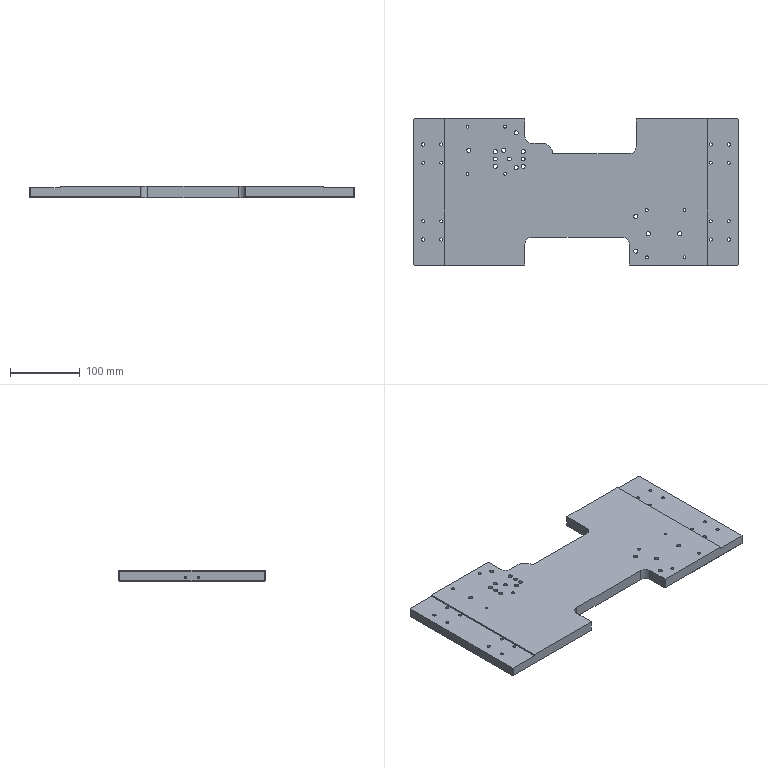NC program | NX | posted with a generic post | part box 467 x 210 x 16 mm
Whole program, first 1630 of 1789 lines:
N10 G17 G21 G94 G90
(FLOOR_WALL , TOOL : D63)
N12 T01 M6
N14 G54
N16 G17 G0 G90 X-271. Y107.997 S6500 M3
N18 G43 Z30. H1
N20 Z3.
N22 G94 G1 Z0. F1250.
N24 X-268.
N26 X268.
N28 Y80.74
N30 X-268.
N32 Y53.484
N34 X268.
N36 Y26.227
N38 X-268.
N40 Y-1.03
N42 X268.
N44 Y-28.287
N46 X-268.
N48 Y-55.543
N50 X268.
N52 Y-82.8
N54 X-268.
N56 X-271.
N58 Z3.
N60 G0 Z30.
N62 M5
(DRILLING_COPY_1 , TOOL : D6A45)
N64 T07 M6
N66 G54
N68 G17 G0 G90 X141.5 Y-65. S3000 M3
N70 G43 Z30. H7
N72 G94 G81 G98 Z-2.1 F200. R3.
N74 X193.5 Y-68.3
N76 X196.5 Y-99.
N78 X225.5
N80 X219.5 Y-68.3
N82 Y-42.3
N84 X225.5 Y-31.
N86 X193.5 Y-42.3
N88 X196.5 Y-31.
N90 X193.5 Y42.3
N92 X219.5
N94 Y68.3
N96 X193.5
N98 X156. Y94.
N100 X154. Y60.
N102 X156. Y26.
N104 X141.5 Y5.
N106 X91.5
N108 X102. Y26.
N110 X116. Y37.
N112 Y47.5
N114 Y58.
N116 X102. Y94.
N118 X86. Y85.
N120 X104. Y60.
N122 X96. Y47.5
N124 X86. Y35.
N126 X76. Y37.
N128 Y47.5
N130 Y58.
N132 X-8.5 Y5.
N134 X-108.5
N136 X-102. Y-26.
N138 X-86. Y-35.
N140 X-104. Y-60.
N142 X-86. Y-85.
N144 X-102. Y-94.
N146 X-156.
N148 X-149. Y-60.
N150 X-156. Y-26.
N152 X-193.5 Y-42.3
N154 Y-68.3
N156 X-219.5
N158 Y-42.3
N160 X-208.5 Y5.
N162 X-219.5 Y42.3
N164 Y68.3
N166 X-193.5
N168 Y42.3
N170 G80
N172 G0 X-193.5 Y42.3 Z30.
N174 M5
(DRILLING_COPY_1_COPY_COPY_COPY_COPY , TOOL : 4.5ZT)
N176 T19 M6
N178 G54
N180 G17 G0 G90 X-193.5 Y-68.3 S2000 M3
N182 G43 Z30. H19
N184 G94 G83 G98 Z-15.852 F150. Q2. R3.
N186 X-219.5
N188 Y-42.3
N190 X-193.5
N192 Y42.3
N194 X-219.5
N196 Y68.3
N198 X-193.5
N200 X193.5
N202 X219.5
N204 Y42.3
N206 X193.5
N208 Y-42.3
N210 Y-68.3
N212 X219.5
N214 Y-42.3
N216 G80
N218 G0 X219.5 Y-42.3 Z30.
N220 M5
(DRILLING_COPY_1_COPY_COPY_1 , TOOL : 5.8ZT)
N222 T18 M6
N224 G54
N226 G17 G0 G90 X-149. Y-60. S2000 M3
N228 G43 Z30. H18
N230 G94 G83 G98 Z-19.242 F120. Q2. R3.
N232 X-104.
N234 X-86. Y-85.
N236 Y-35.
N238 X76. Y37.
N240 X86. Y35.
N242 X76. Y58.
N244 X86. Y85.
N246 X104. Y60.
N248 X116. Y58.
N250 Y37.
N252 X154. Y60.
N254 G80
N256 G0 X154. Y60. Z30.
N258 M5
(DRILLING_COPY_1_COPY_COPY_1_COPY , TOOL : 6.0JD)
N260 T20 M6
N262 G54
N264 G17 G0 G90 X-149. Y-60. S1000 M3
N266 G43 Z30. H20
N268 G94 G85 G98 Z-16.5 F40. R3.
N270 X-104.
N272 X-86. Y-85.
N274 Y-35.
N276 X76. Y37.
N278 X86. Y35.
N280 X76. Y58.
N282 X86. Y85.
N284 X104. Y60.
N286 X116. Y58.
N288 Y37.
N290 X154. Y60.
N292 G80
N294 G0 X154. Y60. Z30.
N296 M5
(DRILLING_COPY_1_COPY_COPY_1_COPY_1 , TOOL : 5.5ZT)
N298 T12 M6
N300 G54
N302 G17 G0 G90 X76. Y47.5 S2000 M3
N304 G43 Z30. H12
N306 G94 G83 G98 Z-19.152 F120. Q2. R3.
N308 X96.
N310 X116.
N312 G80
N314 G0 X116. Y47.5 Z30.
N316 M5
(DRILLING_COPY_1_COPY , TOOL : 4.2ZT)
N318 T14 M6
N320 G54
N322 G17 G0 G90 X102. Y94. S2000 M3
N324 G43 Z30. H14
N326 G94 G83 G98 Z-18.762 F150. Q2. R3.
N328 X156.
N330 Y26.
N332 X102.
N334 X-102. Y-26.
N336 X-156.
N338 Y-94.
N340 X-102.
N342 G80
N344 G0 X-102. Y-94. Z30.
N346 M5
(DRILLING_COPY_1_COPY_COPY_COPY_COPY_COPY , TOOL : 3.3ZT)
N348 T13 M6
N350 G54
N352 G17 G0 G90 X141.5 Y-65. S2000 M3
N354 G43 Z30. H13
N356 G94 G83 G98 Z-11.091 F150. Q2. R3.
N358 X196.5 Y-99. Z-9.091
N360 X225.5
N362 Y-31.
N364 X196.5
N366 X141.5 Y5. Z-11.091
N368 X91.5
N370 X-8.5
N372 X-108.5
N374 X-208.5
N376 G80
N378 G0 X-208.5 Y5. Z30.
N380 M5
(ZLEVEL_PROFILE , TOOL : D10)
N382 T10 M6
N384 G54
N386 G17 G0 G90 X-238.6 Y-46.987 S7000 M3
N388 G43 Z30. H10
N390 Z1.5
N392 G94 G1 Y0. Z-0.963 F1000.
N394 Y104. F3000.
N396 G2 X-237.106 Y107.606 R5.1
N398 G1 X-236.106 Y108.606
N400 G2 X-232.5 Y110.1 R5.1
N402 G1 X-86.5
N404 G2 X-81.4 Y105. R5.1
N406 G1 Y65.
N408 G3 X-76.5 Y60.1 R4.9
N410 G1 X28.401
N412 G2 X29.894 Y63.606 R5.1
N414 G1 X39.894 Y73.606
N416 G2 X43.5 Y75.1 R5.1
N418 G1 X63.5
N420 G3 X68.4 Y80. R4.9
N422 G1 Y105.
N424 G2 X73.5 Y110.1 R5.1
N426 G1 X232.5
N428 G2 X236.106 Y108.606 R5.1
N430 G1 X237.106 Y107.606
N432 G2 X238.6 Y104. R5.1
N434 G1 Y-104.
N436 G2 X237.106 Y-107.606 R5.1
N438 G1 X236.106 Y-108.606
N440 G2 X232.5 Y-110.1 R5.1
N442 G1 X73.5
N444 G2 X68.4 Y-105. R5.1
N446 G1 Y-75.
N448 G3 X63.5 Y-70.1 R4.9
N450 G1 X-66.5
N452 G3 X-71.4 Y-75. R4.9
N454 G1 Y-105.
N456 G2 X-76.5 Y-110.1 R5.1
N458 G1 X-232.5
N460 G2 X-236.106 Y-108.606 R5.1
N462 G1 X-237.106 Y-107.606
N464 G2 X-238.6 Y-104. R5.1
N466 G1 Y0.
N468 Y55.142 Z-1.925
N470 Y104.
N472 G2 X-237.106 Y107.606 R5.1
N474 G1 X-236.106 Y108.606
N476 G2 X-232.5 Y110.1 R5.1
N478 G1 X-86.5
N480 G2 X-81.4 Y105. R5.1
N482 G1 Y65.
N484 G3 X-76.5 Y60.1 R4.9
N486 G1 X28.401
N488 G2 X29.894 Y63.606 R5.1
N490 G1 X39.894 Y73.606
N492 G2 X43.5 Y75.1 R5.1
N494 G1 X63.5
N496 G3 X68.4 Y80. R4.9
N498 G1 Y105.
N500 G2 X73.5 Y110.1 R5.1
N502 G1 X232.5
N504 G2 X236.106 Y108.606 R5.1
N506 G1 X237.106 Y107.606
N508 G2 X238.6 Y104. R5.1
N510 G1 Y-104.
N512 G2 X237.106 Y-107.606 R5.1
N514 G1 X236.106 Y-108.606
N516 G2 X232.5 Y-110.1 R5.1
N518 G1 X73.5
N520 G2 X68.4 Y-105. R5.1
N522 G1 Y-75.
N524 G3 X63.5 Y-70.1 R4.9
N526 G1 X-66.5
N528 G3 X-71.4 Y-75. R4.9
N530 G1 Y-105.
N532 G2 X-76.5 Y-110.1 R5.1
N534 G1 X-232.5
N536 G2 X-236.106 Y-108.606 R5.1
N538 G1 X-237.106 Y-107.606
N540 G2 X-238.6 Y-104. R5.1
N542 G1 Y0.
N544 Y55.142 Z-2.888
N546 Y104.
N548 G2 X-237.106 Y107.606 R5.1
N550 G1 X-236.106 Y108.606
N552 G2 X-232.5 Y110.1 R5.1
N554 G1 X-86.5
N556 G2 X-81.4 Y105. R5.1
N558 G1 Y65.
N560 G3 X-76.5 Y60.1 R4.9
N562 G1 X28.401
N564 G2 X29.894 Y63.606 R5.1
N566 G1 X39.894 Y73.606
N568 G2 X43.5 Y75.1 R5.1
N570 G1 X63.5
N572 G3 X68.4 Y80. R4.9
N574 G1 Y105.
N576 G2 X73.5 Y110.1 R5.1
N578 G1 X232.5
N580 G2 X236.106 Y108.606 R5.1
N582 G1 X237.106 Y107.606
N584 G2 X238.6 Y104. R5.1
N586 G1 Y-104.
N588 G2 X237.106 Y-107.606 R5.1
N590 G1 X236.106 Y-108.606
N592 G2 X232.5 Y-110.1 R5.1
N594 G1 X73.5
N596 G2 X68.4 Y-105. R5.1
N598 G1 Y-75.
N600 G3 X63.5 Y-70.1 R4.9
N602 G1 X-66.5
N604 G3 X-71.4 Y-75. R4.9
N606 G1 Y-105.
N608 G2 X-76.5 Y-110.1 R5.1
N610 G1 X-232.5
N612 G2 X-236.106 Y-108.606 R5.1
N614 G1 X-237.106 Y-107.606
N616 G2 X-238.6 Y-104. R5.1
N618 G1 Y0.
N620 Y55.142 Z-3.85
N622 Y104.
N624 G2 X-237.106 Y107.606 R5.1
N626 G1 X-236.106 Y108.606
N628 G2 X-232.5 Y110.1 R5.1
N630 G1 X-86.5
N632 G2 X-81.4 Y105. R5.1
N634 G1 Y65.
N636 G3 X-76.5 Y60.1 R4.9
N638 G1 X28.401
N640 G2 X29.894 Y63.606 R5.1
N642 G1 X39.894 Y73.606
N644 G2 X43.5 Y75.1 R5.1
N646 G1 X63.5
N648 G3 X68.4 Y80. R4.9
N650 G1 Y105.
N652 G2 X73.5 Y110.1 R5.1
N654 G1 X232.5
N656 G2 X236.106 Y108.606 R5.1
N658 G1 X237.106 Y107.606
N660 G2 X238.6 Y104. R5.1
N662 G1 Y-104.
N664 G2 X237.106 Y-107.606 R5.1
N666 G1 X236.106 Y-108.606
N668 G2 X232.5 Y-110.1 R5.1
N670 G1 X73.5
N672 G2 X68.4 Y-105. R5.1
N674 G1 Y-75.
N676 G3 X63.5 Y-70.1 R4.9
N678 G1 X-66.5
N680 G3 X-71.4 Y-75. R4.9
N682 G1 Y-105.
N684 G2 X-76.5 Y-110.1 R5.1
N686 G1 X-232.5
N688 G2 X-236.106 Y-108.606 R5.1
N690 G1 X-237.106 Y-107.606
N692 G2 X-238.6 Y-104. R5.1
N694 G1 Y0.
N696 Y55.142 Z-4.813
N698 Y104.
N700 G2 X-237.106 Y107.606 R5.1
N702 G1 X-236.106 Y108.606
N704 G2 X-232.5 Y110.1 R5.1
N706 G1 X-86.5
N708 G2 X-81.4 Y105. R5.1
N710 G1 Y65.
N712 G3 X-76.5 Y60.1 R4.9
N714 G1 X28.401
N716 G2 X29.894 Y63.606 R5.1
N718 G1 X39.894 Y73.606
N720 G2 X43.5 Y75.1 R5.1
N722 G1 X63.5
N724 G3 X68.4 Y80. R4.9
N726 G1 Y105.
N728 G2 X73.5 Y110.1 R5.1
N730 G1 X232.5
N732 G2 X236.106 Y108.606 R5.1
N734 G1 X237.106 Y107.606
N736 G2 X238.6 Y104. R5.1
N738 G1 Y-104.
N740 G2 X237.106 Y-107.606 R5.1
N742 G1 X236.106 Y-108.606
N744 G2 X232.5 Y-110.1 R5.1
N746 G1 X73.5
N748 G2 X68.4 Y-105. R5.1
N750 G1 Y-75.
N752 G3 X63.5 Y-70.1 R4.9
N754 G1 X-66.5
N756 G3 X-71.4 Y-75. R4.9
N758 G1 Y-105.
N760 G2 X-76.5 Y-110.1 R5.1
N762 G1 X-232.5
N764 G2 X-236.106 Y-108.606 R5.1
N766 G1 X-237.106 Y-107.606
N768 G2 X-238.6 Y-104. R5.1
N770 G1 Y0.
N772 Y55.142 Z-5.775
N774 Y104.
N776 G2 X-237.106 Y107.606 R5.1
N778 G1 X-236.106 Y108.606
N780 G2 X-232.5 Y110.1 R5.1
N782 G1 X-86.5
N784 G2 X-81.4 Y105. R5.1
N786 G1 Y65.
N788 G3 X-76.5 Y60.1 R4.9
N790 G1 X28.401
N792 G2 X29.894 Y63.606 R5.1
N794 G1 X39.894 Y73.606
N796 G2 X43.5 Y75.1 R5.1
N798 G1 X63.5
N800 G3 X68.4 Y80. R4.9
N802 G1 Y105.
N804 G2 X73.5 Y110.1 R5.1
N806 G1 X232.5
N808 G2 X236.106 Y108.606 R5.1
N810 G1 X237.106 Y107.606
N812 G2 X238.6 Y104. R5.1
N814 G1 Y-104.
N816 G2 X237.106 Y-107.606 R5.1
N818 G1 X236.106 Y-108.606
N820 G2 X232.5 Y-110.1 R5.1
N822 G1 X73.5
N824 G2 X68.4 Y-105. R5.1
N826 G1 Y-75.
N828 G3 X63.5 Y-70.1 R4.9
N830 G1 X-66.5
N832 G3 X-71.4 Y-75. R4.9
N834 G1 Y-105.
N836 G2 X-76.5 Y-110.1 R5.1
N838 G1 X-232.5
N840 G2 X-236.106 Y-108.606 R5.1
N842 G1 X-237.106 Y-107.606
N844 G2 X-238.6 Y-104. R5.1
N846 G1 Y0.
N848 Y55.142 Z-6.738
N850 Y104.
N852 G2 X-237.106 Y107.606 R5.1
N854 G1 X-236.106 Y108.606
N856 G2 X-232.5 Y110.1 R5.1
N858 G1 X-86.5
N860 G2 X-81.4 Y105. R5.1
N862 G1 Y65.
N864 G3 X-76.5 Y60.1 R4.9
N866 G1 X28.401
N868 G2 X29.894 Y63.606 R5.1
N870 G1 X39.894 Y73.606
N872 G2 X43.5 Y75.1 R5.1
N874 G1 X63.5
N876 G3 X68.4 Y80. R4.9
N878 G1 Y105.
N880 G2 X73.5 Y110.1 R5.1
N882 G1 X232.5
N884 G2 X236.106 Y108.606 R5.1
N886 G1 X237.106 Y107.606
N888 G2 X238.6 Y104. R5.1
N890 G1 Y-104.
N892 G2 X237.106 Y-107.606 R5.1
N894 G1 X236.106 Y-108.606
N896 G2 X232.5 Y-110.1 R5.1
N898 G1 X73.5
N900 G2 X68.4 Y-105. R5.1
N902 G1 Y-75.
N904 G3 X63.5 Y-70.1 R4.9
N906 G1 X-66.5
N908 G3 X-71.4 Y-75. R4.9
N910 G1 Y-105.
N912 G2 X-76.5 Y-110.1 R5.1
N914 G1 X-232.5
N916 G2 X-236.106 Y-108.606 R5.1
N918 G1 X-237.106 Y-107.606
N920 G2 X-238.6 Y-104. R5.1
N922 G1 Y0.
N924 Y55.142 Z-7.7
N926 Y104.
N928 G2 X-237.106 Y107.606 R5.1
N930 G1 X-236.106 Y108.606
N932 G2 X-232.5 Y110.1 R5.1
N934 G1 X-86.5
N936 G2 X-81.4 Y105. R5.1
N938 G1 Y65.
N940 G3 X-76.5 Y60.1 R4.9
N942 G1 X28.401
N944 G2 X29.894 Y63.606 R5.1
N946 G1 X39.894 Y73.606
N948 G2 X43.5 Y75.1 R5.1
N950 G1 X63.5
N952 G3 X68.4 Y80. R4.9
N954 G1 Y105.
N956 G2 X73.5 Y110.1 R5.1
N958 G1 X232.5
N960 G2 X236.106 Y108.606 R5.1
N962 G1 X237.106 Y107.606
N964 G2 X238.6 Y104. R5.1
N966 G1 Y-104.
N968 G2 X237.106 Y-107.606 R5.1
N970 G1 X236.106 Y-108.606
N972 G2 X232.5 Y-110.1 R5.1
N974 G1 X73.5
N976 G2 X68.4 Y-105. R5.1
N978 G1 Y-75.
N980 G3 X63.5 Y-70.1 R4.9
N982 G1 X-66.5
N984 G3 X-71.4 Y-75. R4.9
N986 G1 Y-105.
N988 G2 X-76.5 Y-110.1 R5.1
N990 G1 X-232.5
N992 G2 X-236.106 Y-108.606 R5.1
N994 G1 X-237.106 Y-107.606
N996 G2 X-238.6 Y-104. R5.1
N998 G1 Y0.
N1000 Y55.142 Z-8.663
N1002 Y104.
N1004 G2 X-237.106 Y107.606 R5.1
N1006 G1 X-236.106 Y108.606
N1008 G2 X-232.5 Y110.1 R5.1
N1010 G1 X-86.5
N1012 G2 X-81.4 Y105. R5.1
N1014 G1 Y65.
N1016 G3 X-76.5 Y60.1 R4.9
N1018 G1 X28.401
N1020 G2 X29.894 Y63.606 R5.1
N1022 G1 X39.894 Y73.606
N1024 G2 X43.5 Y75.1 R5.1
N1026 G1 X63.5
N1028 G3 X68.4 Y80. R4.9
N1030 G1 Y105.
N1032 G2 X73.5 Y110.1 R5.1
N1034 G1 X232.5
N1036 G2 X236.106 Y108.606 R5.1
N1038 G1 X237.106 Y107.606
N1040 G2 X238.6 Y104. R5.1
N1042 G1 Y-104.
N1044 G2 X237.106 Y-107.606 R5.1
N1046 G1 X236.106 Y-108.606
N1048 G2 X232.5 Y-110.1 R5.1
N1050 G1 X73.5
N1052 G2 X68.4 Y-105. R5.1
N1054 G1 Y-75.
N1056 G3 X63.5 Y-70.1 R4.9
N1058 G1 X-66.5
N1060 G3 X-71.4 Y-75. R4.9
N1062 G1 Y-105.
N1064 G2 X-76.5 Y-110.1 R5.1
N1066 G1 X-232.5
N1068 G2 X-236.106 Y-108.606 R5.1
N1070 G1 X-237.106 Y-107.606
N1072 G2 X-238.6 Y-104. R5.1
N1074 G1 Y0.
N1076 Y55.142 Z-9.625
N1078 Y104.
N1080 G2 X-237.106 Y107.606 R5.1
N1082 G1 X-236.106 Y108.606
N1084 G2 X-232.5 Y110.1 R5.1
N1086 G1 X-86.5
N1088 G2 X-81.4 Y105. R5.1
N1090 G1 Y65.
N1092 G3 X-76.5 Y60.1 R4.9
N1094 G1 X28.401
N1096 G2 X29.894 Y63.606 R5.1
N1098 G1 X39.894 Y73.606
N1100 G2 X43.5 Y75.1 R5.1
N1102 G1 X63.5
N1104 G3 X68.4 Y80. R4.9
N1106 G1 Y105.
N1108 G2 X73.5 Y110.1 R5.1
N1110 G1 X232.5
N1112 G2 X236.106 Y108.606 R5.1
N1114 G1 X237.106 Y107.606
N1116 G2 X238.6 Y104. R5.1
N1118 G1 Y-104.
N1120 G2 X237.106 Y-107.606 R5.1
N1122 G1 X236.106 Y-108.606
N1124 G2 X232.5 Y-110.1 R5.1
N1126 G1 X73.5
N1128 G2 X68.4 Y-105. R5.1
N1130 G1 Y-75.
N1132 G3 X63.5 Y-70.1 R4.9
N1134 G1 X-66.5
N1136 G3 X-71.4 Y-75. R4.9
N1138 G1 Y-105.
N1140 G2 X-76.5 Y-110.1 R5.1
N1142 G1 X-232.5
N1144 G2 X-236.106 Y-108.606 R5.1
N1146 G1 X-237.106 Y-107.606
N1148 G2 X-238.6 Y-104. R5.1
N1150 G1 Y0.
N1152 Y55.142 Z-10.588
N1154 Y104.
N1156 G2 X-237.106 Y107.606 R5.1
N1158 G1 X-236.106 Y108.606
N1160 G2 X-232.5 Y110.1 R5.1
N1162 G1 X-86.5
N1164 G2 X-81.4 Y105. R5.1
N1166 G1 Y65.
N1168 G3 X-76.5 Y60.1 R4.9
N1170 G1 X28.401
N1172 G2 X29.894 Y63.606 R5.1
N1174 G1 X39.894 Y73.606
N1176 G2 X43.5 Y75.1 R5.1
N1178 G1 X63.5
N1180 G3 X68.4 Y80. R4.9
N1182 G1 Y105.
N1184 G2 X73.5 Y110.1 R5.1
N1186 G1 X232.5
N1188 G2 X236.106 Y108.606 R5.1
N1190 G1 X237.106 Y107.606
N1192 G2 X238.6 Y104. R5.1
N1194 G1 Y-104.
N1196 G2 X237.106 Y-107.606 R5.1
N1198 G1 X236.106 Y-108.606
N1200 G2 X232.5 Y-110.1 R5.1
N1202 G1 X73.5
N1204 G2 X68.4 Y-105. R5.1
N1206 G1 Y-75.
N1208 G3 X63.5 Y-70.1 R4.9
N1210 G1 X-66.5
N1212 G3 X-71.4 Y-75. R4.9
N1214 G1 Y-105.
N1216 G2 X-76.5 Y-110.1 R5.1
N1218 G1 X-232.5
N1220 G2 X-236.106 Y-108.606 R5.1
N1222 G1 X-237.106 Y-107.606
N1224 G2 X-238.6 Y-104. R5.1
N1226 G1 Y0.
N1228 Y55.142 Z-11.55
N1230 Y104.
N1232 G2 X-237.106 Y107.606 R5.1
N1234 G1 X-236.106 Y108.606
N1236 G2 X-232.5 Y110.1 R5.1
N1238 G1 X-86.5
N1240 G2 X-81.4 Y105. R5.1
N1242 G1 Y65.
N1244 G3 X-76.5 Y60.1 R4.9
N1246 G1 X28.401
N1248 G2 X29.894 Y63.606 R5.1
N1250 G1 X39.894 Y73.606
N1252 G2 X43.5 Y75.1 R5.1
N1254 G1 X63.5
N1256 G3 X68.4 Y80. R4.9
N1258 G1 Y105.
N1260 G2 X73.5 Y110.1 R5.1
N1262 G1 X232.5
N1264 G2 X236.106 Y108.606 R5.1
N1266 G1 X237.106 Y107.606
N1268 G2 X238.6 Y104. R5.1
N1270 G1 Y-104.
N1272 G2 X237.106 Y-107.606 R5.1
N1274 G1 X236.106 Y-108.606
N1276 G2 X232.5 Y-110.1 R5.1
N1278 G1 X73.5
N1280 G2 X68.4 Y-105. R5.1
N1282 G1 Y-75.
N1284 G3 X63.5 Y-70.1 R4.9
N1286 G1 X-66.5
N1288 G3 X-71.4 Y-75. R4.9
N1290 G1 Y-105.
N1292 G2 X-76.5 Y-110.1 R5.1
N1294 G1 X-232.5
N1296 G2 X-236.106 Y-108.606 R5.1
N1298 G1 X-237.106 Y-107.606
N1300 G2 X-238.6 Y-104. R5.1
N1302 G1 Y0.
N1304 Y55.142 Z-12.513
N1306 Y104.
N1308 G2 X-237.106 Y107.606 R5.1
N1310 G1 X-236.106 Y108.606
N1312 G2 X-232.5 Y110.1 R5.1
N1314 G1 X-86.5
N1316 G2 X-81.4 Y105. R5.1
N1318 G1 Y65.
N1320 G3 X-76.5 Y60.1 R4.9
N1322 G1 X28.401
N1324 G2 X29.894 Y63.606 R5.1
N1326 G1 X39.894 Y73.606
N1328 G2 X43.5 Y75.1 R5.1
N1330 G1 X63.5
N1332 G3 X68.4 Y80. R4.9
N1334 G1 Y105.
N1336 G2 X73.5 Y110.1 R5.1
N1338 G1 X232.5
N1340 G2 X236.106 Y108.606 R5.1
N1342 G1 X237.106 Y107.606
N1344 G2 X238.6 Y104. R5.1
N1346 G1 Y-104.
N1348 G2 X237.106 Y-107.606 R5.1
N1350 G1 X236.106 Y-108.606
N1352 G2 X232.5 Y-110.1 R5.1
N1354 G1 X73.5
N1356 G2 X68.4 Y-105. R5.1
N1358 G1 Y-75.
N1360 G3 X63.5 Y-70.1 R4.9
N1362 G1 X-66.5
N1364 G3 X-71.4 Y-75. R4.9
N1366 G1 Y-105.
N1368 G2 X-76.5 Y-110.1 R5.1
N1370 G1 X-232.5
N1372 G2 X-236.106 Y-108.606 R5.1
N1374 G1 X-237.106 Y-107.606
N1376 G2 X-238.6 Y-104. R5.1
N1378 G1 Y0.
N1380 Y55.142 Z-13.475
N1382 Y104.
N1384 G2 X-237.106 Y107.606 R5.1
N1386 G1 X-236.106 Y108.606
N1388 G2 X-232.5 Y110.1 R5.1
N1390 G1 X-86.5
N1392 G2 X-81.4 Y105. R5.1
N1394 G1 Y65.
N1396 G3 X-76.5 Y60.1 R4.9
N1398 G1 X28.401
N1400 G2 X29.894 Y63.606 R5.1
N1402 G1 X39.894 Y73.606
N1404 G2 X43.5 Y75.1 R5.1
N1406 G1 X63.5
N1408 G3 X68.4 Y80. R4.9
N1410 G1 Y105.
N1412 G2 X73.5 Y110.1 R5.1
N1414 G1 X232.5
N1416 G2 X236.106 Y108.606 R5.1
N1418 G1 X237.106 Y107.606
N1420 G2 X238.6 Y104. R5.1
N1422 G1 Y-104.
N1424 G2 X237.106 Y-107.606 R5.1
N1426 G1 X236.106 Y-108.606
N1428 G2 X232.5 Y-110.1 R5.1
N1430 G1 X73.5
N1432 G2 X68.4 Y-105. R5.1
N1434 G1 Y-75.
N1436 G3 X63.5 Y-70.1 R4.9
N1438 G1 X-66.5
N1440 G3 X-71.4 Y-75. R4.9
N1442 G1 Y-105.
N1444 G2 X-76.5 Y-110.1 R5.1
N1446 G1 X-232.5
N1448 G2 X-236.106 Y-108.606 R5.1
N1450 G1 X-237.106 Y-107.606
N1452 G2 X-238.6 Y-104. R5.1
N1454 G1 Y0.
N1456 Y55.142 Z-14.438
N1458 Y104.
N1460 G2 X-237.106 Y107.606 R5.1
N1462 G1 X-236.106 Y108.606
N1464 G2 X-232.5 Y110.1 R5.1
N1466 G1 X-86.5
N1468 G2 X-81.4 Y105. R5.1
N1470 G1 Y65.
N1472 G3 X-76.5 Y60.1 R4.9
N1474 G1 X28.401
N1476 G2 X29.894 Y63.606 R5.1
N1478 G1 X39.894 Y73.606
N1480 G2 X43.5 Y75.1 R5.1
N1482 G1 X63.5
N1484 G3 X68.4 Y80. R4.9
N1486 G1 Y105.
N1488 G2 X73.5 Y110.1 R5.1
N1490 G1 X232.5
N1492 G2 X236.106 Y108.606 R5.1
N1494 G1 X237.106 Y107.606
N1496 G2 X238.6 Y104. R5.1
N1498 G1 Y-104.
N1500 G2 X237.106 Y-107.606 R5.1
N1502 G1 X236.106 Y-108.606
N1504 G2 X232.5 Y-110.1 R5.1
N1506 G1 X73.5
N1508 G2 X68.4 Y-105. R5.1
N1510 G1 Y-75.
N1512 G3 X63.5 Y-70.1 R4.9
N1514 G1 X-66.5
N1516 G3 X-71.4 Y-75. R4.9
N1518 G1 Y-105.
N1520 G2 X-76.5 Y-110.1 R5.1
N1522 G1 X-232.5
N1524 G2 X-236.106 Y-108.606 R5.1
N1526 G1 X-237.106 Y-107.606
N1528 G2 X-238.6 Y-104. R5.1
N1530 G1 Y0.
N1532 Y55.142 Z-15.4
N1534 Y104.
N1536 G2 X-237.106 Y107.606 R5.1
N1538 G1 X-236.106 Y108.606
N1540 G2 X-232.5 Y110.1 R5.1
N1542 G1 X-86.5
N1544 G2 X-81.4 Y105. R5.1
N1546 G1 Y65.
N1548 G3 X-76.5 Y60.1 R4.9
N1550 G1 X28.401
N1552 G2 X29.894 Y63.606 R5.1
N1554 G1 X39.894 Y73.606
N1556 G2 X43.5 Y75.1 R5.1
N1558 G1 X63.5
N1560 G3 X68.4 Y80. R4.9
N1562 G1 Y105.
N1564 G2 X73.5 Y110.1 R5.1
N1566 G1 X232.5
N1568 G2 X236.106 Y108.606 R5.1
N1570 G1 X237.106 Y107.606
N1572 G2 X238.6 Y104. R5.1
N1574 G1 Y-104.
N1576 G2 X237.106 Y-107.606 R5.1
N1578 G1 X236.106 Y-108.606
N1580 G2 X232.5 Y-110.1 R5.1
N1582 G1 X73.5
N1584 G2 X68.4 Y-105. R5.1
N1586 G1 Y-75.
N1588 G3 X63.5 Y-70.1 R4.9
N1590 G1 X-66.5
N1592 G3 X-71.4 Y-75. R4.9
N1594 G1 Y-105.
N1596 G2 X-76.5 Y-110.1 R5.1
N1598 G1 X-232.5
N1600 G2 X-236.106 Y-108.606 R5.1
N1602 G1 X-237.106 Y-107.606
N1604 G2 X-238.6 Y-104. R5.1
N1606 G1 Y55.142
N1608 Z-13.9
N1610 G0 Z30.
N1612 M5
(HOLE_MILLING , TOOL : D6)
N1614 T06 M6
N1616 G54
N1618 G17 G0 G90 X-219.5 Y68.3 S7000 M3
N1620 G43 Z30. H6
N1622 Z0.5
N1624 G94 G3 X-220. Y68.8 R0.5 F1500.
N1626 X-220.5 Y68.3 R0.5
N1628 X-220.5 Y68.3 Z0. I1. J0.
N1630 X-220.5 Y68.3 Z-0.5 I1. J0.
N1632 X-220.5 Y68.3 Z-1. I1. J0.
N1634 X-220.5 Y68.3 Z-1.5 I1. J0.
N1636 X-220.5 Y68.3 Z-2. I1. J0.
N1638 X-220.5 Y68.3 Z-2.5 I1. J0.
N1640 X-220.5 Y68.3 Z-3. I1. J0.
N1642 X-220.5 Y68.3 Z-3.5 I1. J0.
N1644 X-220.5 Y68.3 Z-4. I1. J0.
N1646 X-219.809 Y69.251 Z-4.4 R-1.
N1648 X-220.451 Y67.991 R1.
N1650 X-219.809 Y69.251 R-1.
N1652 X-220.13 Y68.621 R0.5
N1654 X-219.5 Y68.3 R0.5
N1656 G0 Z30.
N1658 X-193.5
N1660 Z0.5
N1662 G3 X-194. Y68.8 R0.5
N1664 X-194.5 Y68.3 R0.5
N1666 X-194.5 Y68.3 Z0. I1. J0.
N1668 X-194.5 Y68.3 Z-0.5 I1. J0.
N1670 X-194.5 Y68.3 Z-1. I1. J0.
N1672 X-194.5 Y68.3 Z-1.5 I1. J0.
N1674 X-194.5 Y68.3 Z-2. I1. J0.
N1676 X-194.5 Y68.3 Z-2.5 I1. J0.
N1678 X-194.5 Y68.3 Z-3. I1. J0.
N1680 X-194.5 Y68.3 Z-3.5 I1. J0.
N1682 X-194.5 Y68.3 Z-4. I1. J0.
N1684 X-193.809 Y69.251 Z-4.4 R-1.
N1686 X-194.451 Y67.991 R1.
N1688 X-193.809 Y69.251 R-1.
N1690 X-194.13 Y68.621 R0.5
N1692 X-193.5 Y68.3 R0.5
N1694 G0 Z30.
N1696 Y42.3
N1698 Z0.5
N1700 G3 X-194. Y42.8 R0.5
N1702 X-194.5 Y42.3 R0.5
N1704 X-194.5 Y42.3 Z0. I1. J0.
N1706 X-194.5 Y42.3 Z-0.5 I1. J0.
N1708 X-194.5 Y42.3 Z-1. I1. J0.
N1710 X-194.5 Y42.3 Z-1.5 I1. J0.
N1712 X-194.5 Y42.3 Z-2. I1. J0.
N1714 X-194.5 Y42.3 Z-2.5 I1. J0.
N1716 X-194.5 Y42.3 Z-3. I1. J0.
N1718 X-194.5 Y42.3 Z-3.5 I1. J0.
N1720 X-194.5 Y42.3 Z-4. I1. J0.
N1722 X-193.809 Y43.251 Z-4.4 R-1.
N1724 X-194.451 Y41.991 R1.
N1726 X-193.809 Y43.251 R-1.
N1728 X-194.13 Y42.621 R0.5
N1730 X-193.5 Y42.3 R0.5
N1732 G0 Z30.
N1734 X-219.5
N1736 Z0.5
N1738 G3 X-220. Y42.8 R0.5
N1740 X-220.5 Y42.3 R0.5
N1742 X-220.5 Y42.3 Z0. I1. J0.
N1744 X-220.5 Y42.3 Z-0.5 I1. J0.
N1746 X-220.5 Y42.3 Z-1. I1. J0.
N1748 X-220.5 Y42.3 Z-1.5 I1. J0.
N1750 X-220.5 Y42.3 Z-2. I1. J0.
N1752 X-220.5 Y42.3 Z-2.5 I1. J0.
N1754 X-220.5 Y42.3 Z-3. I1. J0.
N1756 X-220.5 Y42.3 Z-3.5 I1. J0.
N1758 X-220.5 Y42.3 Z-4. I1. J0.
N1760 X-219.809 Y43.251 Z-4.4 R-1.
N1762 X-220.451 Y41.991 R1.
N1764 X-219.809 Y43.251 R-1.
N1766 X-220.13 Y42.621 R0.5
N1768 X-219.5 Y42.3 R0.5
N1770 G0 Z30.
N1772 Y-42.3
N1774 Z0.5
N1776 G3 X-220. Y-41.8 R0.5
N1778 X-220.5 Y-42.3 R0.5
N1780 X-220.5 Y-42.3 Z0. I1. J0.
N1782 X-220.5 Y-42.3 Z-0.5 I1. J0.
N1784 X-220.5 Y-42.3 Z-1. I1. J0.
N1786 X-220.5 Y-42.3 Z-1.5 I1. J0.
N1788 X-220.5 Y-42.3 Z-2. I1. J0.
N1790 X-220.5 Y-42.3 Z-2.5 I1. J0.
N1792 X-220.5 Y-42.3 Z-3. I1. J0.
N1794 X-220.5 Y-42.3 Z-3.5 I1. J0.
N1796 X-220.5 Y-42.3 Z-4. I1. J0.
N1798 X-219.809 Y-41.349 Z-4.4 R-1.
N1800 X-220.451 Y-42.609 R1.
N1802 X-219.809 Y-41.349 R-1.
N1804 X-220.13 Y-41.979 R0.5
N1806 X-219.5 Y-42.3 R0.5
N1808 G0 Z30.
N1810 Y-68.3
N1812 Z0.5
N1814 G3 X-220. Y-67.8 R0.5
N1816 X-220.5 Y-68.3 R0.5
N1818 X-220.5 Y-68.3 Z0. I1. J0.
N1820 X-220.5 Y-68.3 Z-0.5 I1. J0.
N1822 X-220.5 Y-68.3 Z-1. I1. J0.
N1824 X-220.5 Y-68.3 Z-1.5 I1. J0.
N1826 X-220.5 Y-68.3 Z-2. I1. J0.
N1828 X-220.5 Y-68.3 Z-2.5 I1. J0.
N1830 X-220.5 Y-68.3 Z-3. I1. J0.
N1832 X-220.5 Y-68.3 Z-3.5 I1. J0.
N1834 X-220.5 Y-68.3 Z-4. I1. J0.
N1836 X-219.809 Y-67.349 Z-4.4 R-1.
N1838 X-220.451 Y-68.609 R1.
N1840 X-219.809 Y-67.349 R-1.
N1842 X-220.13 Y-67.979 R0.5
N1844 X-219.5 Y-68.3 R0.5
N1846 G0 Z30.
N1848 X-193.5
N1850 Z0.5
N1852 G3 X-194. Y-67.8 R0.5
N1854 X-194.5 Y-68.3 R0.5
N1856 X-194.5 Y-68.3 Z0. I1. J0.
N1858 X-194.5 Y-68.3 Z-0.5 I1. J0.
N1860 X-194.5 Y-68.3 Z-1. I1. J0.
N1862 X-194.5 Y-68.3 Z-1.5 I1. J0.
N1864 X-194.5 Y-68.3 Z-2. I1. J0.
N1866 X-194.5 Y-68.3 Z-2.5 I1. J0.
N1868 X-194.5 Y-68.3 Z-3. I1. J0.
N1870 X-194.5 Y-68.3 Z-3.5 I1. J0.
N1872 X-194.5 Y-68.3 Z-4. I1. J0.
N1874 X-193.809 Y-67.349 Z-4.4 R-1.
N1876 X-194.451 Y-68.609 R1.
N1878 X-193.809 Y-67.349 R-1.
N1880 X-194.13 Y-67.979 R0.5
N1882 X-193.5 Y-68.3 R0.5
N1884 G0 Z30.
N1886 Y-42.3
N1888 Z0.5
N1890 G3 X-194. Y-41.8 R0.5
N1892 X-194.5 Y-42.3 R0.5
N1894 X-194.5 Y-42.3 Z0. I1. J0.
N1896 X-194.5 Y-42.3 Z-0.5 I1. J0.
N1898 X-194.5 Y-42.3 Z-1. I1. J0.
N1900 X-194.5 Y-42.3 Z-1.5 I1. J0.
N1902 X-194.5 Y-42.3 Z-2. I1. J0.
N1904 X-194.5 Y-42.3 Z-2.5 I1. J0.
N1906 X-194.5 Y-42.3 Z-3. I1. J0.
N1908 X-194.5 Y-42.3 Z-3.5 I1. J0.
N1910 X-194.5 Y-42.3 Z-4. I1. J0.
N1912 X-193.809 Y-41.349 Z-4.4 R-1.
N1914 X-194.451 Y-42.609 R1.
N1916 X-193.809 Y-41.349 R-1.
N1918 X-194.13 Y-41.979 R0.5
N1920 X-193.5 Y-42.3 R0.5
N1922 G0 Z30.
N1924 X76. Y47.5
N1926 Z0.5
N1928 G3 X75. Y48.5 R1.
N1930 X74. Y47.5 R1.
N1932 X74. Y47.5 Z0. I2. J0.
N1934 X74. Y47.5 Z-0.5 I2. J0.
N1936 X74. Y47.5 Z-1. I2. J0.
N1938 X74. Y47.5 Z-1.5 I2. J0.
N1940 X74. Y47.5 Z-2. I2. J0.
N1942 X74. Y47.5 Z-2.5 I2. J0.
N1944 X74. Y47.5 Z-3. I2. J0.
N1946 X74. Y47.5 Z-3.5 I2. J0.
N1948 X74. Y47.5 Z-4. I2. J0.
N1950 X75.382 Y49.402 Z-4.4 R-2.
N1952 X74.098 Y46.882 R2.
N1954 X75.382 Y49.402 R-2.
N1956 X74.74 Y48.142 R1.
N1958 X76. Y47.5 R1.
N1960 G0 Z30.
N1962 X96.
N1964 Z0.5
N1966 G3 X95. Y48.5 R1.
N1968 X94. Y47.5 R1.
N1970 X94. Y47.5 Z0. I2. J0.
N1972 X94. Y47.5 Z-0.5 I2. J0.
N1974 X94. Y47.5 Z-1. I2. J0.
N1976 X94. Y47.5 Z-1.5 I2. J0.
N1978 X94. Y47.5 Z-2. I2. J0.
N1980 X94. Y47.5 Z-2.5 I2. J0.
N1982 X94. Y47.5 Z-3. I2. J0.
N1984 X94. Y47.5 Z-3.5 I2. J0.
N1986 X94. Y47.5 Z-4. I2. J0.
N1988 X95.382 Y49.402 Z-4.4 R-2.
N1990 X94.098 Y46.882 R2.
N1992 X95.382 Y49.402 R-2.
N1994 X94.74 Y48.142 R1.
N1996 X96. Y47.5 R1.
N1998 G0 Z30.
N2000 X116.
N2002 Z0.5
N2004 G3 X115. Y48.5 R1.
N2006 X114. Y47.5 R1.
N2008 X114. Y47.5 Z0. I2. J0.
N2010 X114. Y47.5 Z-0.5 I2. J0.
N2012 X114. Y47.5 Z-1. I2. J0.
N2014 X114. Y47.5 Z-1.5 I2. J0.
N2016 X114. Y47.5 Z-2. I2. J0.
N2018 X114. Y47.5 Z-2.5 I2. J0.
N2020 X114. Y47.5 Z-3. I2. J0.
N2022 X114. Y47.5 Z-3.5 I2. J0.
N2024 X114. Y47.5 Z-4. I2. J0.
N2026 X115.382 Y49.402 Z-4.4 R-2.
N2028 X114.098 Y46.882 R2.
N2030 X115.382 Y49.402 R-2.
N2032 X114.74 Y48.142 R1.
N2034 X116. Y47.5 R1.
N2036 G0 Z30.
N2038 X193.5 Y42.3
N2040 Z0.5
N2042 G3 X193. Y42.8 R0.5
N2044 X192.5 Y42.3 R0.5
N2046 X192.5 Y42.3 Z0. I1. J0.
N2048 X192.5 Y42.3 Z-0.5 I1. J0.
N2050 X192.5 Y42.3 Z-1. I1. J0.
N2052 X192.5 Y42.3 Z-1.5 I1. J0.
N2054 X192.5 Y42.3 Z-2. I1. J0.
N2056 X192.5 Y42.3 Z-2.5 I1. J0.
N2058 X192.5 Y42.3 Z-3. I1. J0.
N2060 X192.5 Y42.3 Z-3.5 I1. J0.
N2062 X192.5 Y42.3 Z-4. I1. J0.
N2064 X193.191 Y43.251 Z-4.4 R-1.
N2066 X192.549 Y41.991 R1.
N2068 X193.191 Y43.251 R-1.
N2070 X192.87 Y42.621 R0.5
N2072 X193.5 Y42.3 R0.5
N2074 G0 Z30.
N2076 Y68.3
N2078 Z0.5
N2080 G3 X193. Y68.8 R0.5
N2082 X192.5 Y68.3 R0.5
N2084 X192.5 Y68.3 Z0. I1. J0.
N2086 X192.5 Y68.3 Z-0.5 I1. J0.
N2088 X192.5 Y68.3 Z-1. I1. J0.
N2090 X192.5 Y68.3 Z-1.5 I1. J0.
N2092 X192.5 Y68.3 Z-2. I1. J0.
N2094 X192.5 Y68.3 Z-2.5 I1. J0.
N2096 X192.5 Y68.3 Z-3. I1. J0.
N2098 X192.5 Y68.3 Z-3.5 I1. J0.
N2100 X192.5 Y68.3 Z-4. I1. J0.
N2102 X193.191 Y69.251 Z-4.4 R-1.
N2104 X192.549 Y67.991 R1.
N2106 X193.191 Y69.251 R-1.
N2108 X192.87 Y68.621 R0.5
N2110 X193.5 Y68.3 R0.5
N2112 G0 Z30.
N2114 X219.5
N2116 Z0.5
N2118 G3 X219. Y68.8 R0.5
N2120 X218.5 Y68.3 R0.5
N2122 X218.5 Y68.3 Z0. I1. J0.
N2124 X218.5 Y68.3 Z-0.5 I1. J0.
N2126 X218.5 Y68.3 Z-1. I1. J0.
N2128 X218.5 Y68.3 Z-1.5 I1. J0.
N2130 X218.5 Y68.3 Z-2. I1. J0.
N2132 X218.5 Y68.3 Z-2.5 I1. J0.
N2134 X218.5 Y68.3 Z-3. I1. J0.
N2136 X218.5 Y68.3 Z-3.5 I1. J0.
N2138 X218.5 Y68.3 Z-4. I1. J0.
N2140 X219.191 Y69.251 Z-4.4 R-1.
N2142 X218.549 Y67.991 R1.
N2144 X219.191 Y69.251 R-1.
N2146 X218.87 Y68.621 R0.5
N2148 X219.5 Y68.3 R0.5
N2150 G0 Z30.
N2152 Y42.3
N2154 Z0.5
N2156 G3 X219. Y42.8 R0.5
N2158 X218.5 Y42.3 R0.5
N2160 X218.5 Y42.3 Z0. I1. J0.
N2162 X218.5 Y42.3 Z-0.5 I1. J0.
N2164 X218.5 Y42.3 Z-1. I1. J0.
N2166 X218.5 Y42.3 Z-1.5 I1. J0.
N2168 X218.5 Y42.3 Z-2. I1. J0.
N2170 X218.5 Y42.3 Z-2.5 I1. J0.
N2172 X218.5 Y42.3 Z-3. I1. J0.
N2174 X218.5 Y42.3 Z-3.5 I1. J0.
N2176 X218.5 Y42.3 Z-4. I1. J0.
N2178 X219.191 Y43.251 Z-4.4 R-1.
N2180 X218.549 Y41.991 R1.
N2182 X219.191 Y43.251 R-1.
N2184 X218.87 Y42.621 R0.5
N2186 X219.5 Y42.3 R0.5
N2188 G0 Z30.
N2190 Y-42.3
N2192 Z0.5
N2194 G3 X219. Y-41.8 R0.5
N2196 X218.5 Y-42.3 R0.5
N2198 X218.5 Y-42.3 Z0. I1. J0.
N2200 X218.5 Y-42.3 Z-0.5 I1. J0.
N2202 X218.5 Y-42.3 Z-1. I1. J0.
N2204 X218.5 Y-42.3 Z-1.5 I1. J0.
N2206 X218.5 Y-42.3 Z-2. I1. J0.
N2208 X218.5 Y-42.3 Z-2.5 I1. J0.
N2210 X218.5 Y-42.3 Z-3. I1. J0.
N2212 X218.5 Y-42.3 Z-3.5 I1. J0.
N2214 X218.5 Y-42.3 Z-4. I1. J0.
N2216 X219.191 Y-41.349 Z-4.4 R-1.
N2218 X218.549 Y-42.609 R1.
N2220 X219.191 Y-41.349 R-1.
N2222 X218.87 Y-41.979 R0.5
N2224 X219.5 Y-42.3 R0.5
N2226 G0 Z30.
N2228 Y-68.3
N2230 Z0.5
N2232 G3 X219. Y-67.8 R0.5
N2234 X218.5 Y-68.3 R0.5
N2236 X218.5 Y-68.3 Z0. I1. J0.
N2238 X218.5 Y-68.3 Z-0.5 I1. J0.
N2240 X218.5 Y-68.3 Z-1. I1. J0.
N2242 X218.5 Y-68.3 Z-1.5 I1. J0.
N2244 X218.5 Y-68.3 Z-2. I1. J0.
N2246 X218.5 Y-68.3 Z-2.5 I1. J0.
N2248 X218.5 Y-68.3 Z-3. I1. J0.
N2250 X218.5 Y-68.3 Z-3.5 I1. J0.
N2252 X218.5 Y-68.3 Z-4. I1. J0.
N2254 X219.191 Y-67.349 Z-4.4 R-1.
N2256 X218.549 Y-68.609 R1.
N2258 X219.191 Y-67.349 R-1.
N2260 X218.87 Y-67.979 R0.5
N2262 X219.5 Y-68.3 R0.5
N2264 G0 Z30.
N2266 X193.5
N2268 Z0.5
N2270 G3 X193. Y-67.8 R0.5
N2272 X192.5 Y-68.3 R0.5
N2274 X192.5 Y-68.3 Z0. I1. J0.
N2276 X192.5 Y-68.3 Z-0.5 I1. J0.
N2278 X192.5 Y-68.3 Z-1. I1. J0.
N2280 X192.5 Y-68.3 Z-1.5 I1. J0.
N2282 X192.5 Y-68.3 Z-2. I1. J0.
N2284 X192.5 Y-68.3 Z-2.5 I1. J0.
N2286 X192.5 Y-68.3 Z-3. I1. J0.
N2288 X192.5 Y-68.3 Z-3.5 I1. J0.
N2290 X192.5 Y-68.3 Z-4. I1. J0.
N2292 X193.191 Y-67.349 Z-4.4 R-1.
N2294 X192.549 Y-68.609 R1.
N2296 X193.191 Y-67.349 R-1.
N2298 X192.87 Y-67.979 R0.5
N2300 X193.5 Y-68.3 R0.5
N2302 G0 Z30.
N2304 Y-42.3
N2306 Z0.5
N2308 G3 X193. Y-41.8 R0.5
N2310 X192.5 Y-42.3 R0.5
N2312 X192.5 Y-42.3 Z0. I1. J0.
N2314 X192.5 Y-42.3 Z-0.5 I1. J0.
N2316 X192.5 Y-42.3 Z-1. I1. J0.
N2318 X192.5 Y-42.3 Z-1.5 I1. J0.
N2320 X192.5 Y-42.3 Z-2. I1. J0.
N2322 X192.5 Y-42.3 Z-2.5 I1. J0.
N2324 X192.5 Y-42.3 Z-3. I1. J0.
N2326 X192.5 Y-42.3 Z-3.5 I1. J0.
N2328 X192.5 Y-42.3 Z-4. I1. J0.
N2330 X193.191 Y-41.349 Z-4.4 R-1.
N2332 X192.549 Y-42.609 R1.
N2334 X193.191 Y-41.349 R-1.
N2336 X192.87 Y-41.979 R0.5
N2338 X193.5 Y-42.3 R0.5
N2340 G0 Z30.
N2342 M5
(ZLEVEL_PROFILE_COPY_1_COPY_COPY_COPY_COPY_2_COPY , TOOL : D6A45)
N2344 T07 M6
N2346 G54
N2348 G17 G0 G90 X76.155 Y58.395 S7000 M3
N2350 G43 Z30. H7
N2352 Z-1.5
N2354 G94 G1 X76.52 Y59.324 F1000.
N2356 G3 X76. Y59.624 R0.6
N2358 X74.376 Y58. R1.624
N2360 X76. Y59.624 R-1.624
N2362 X75.48 Y59.324 R0.6
N2364 G1 X75.845 Y58.395
N2366 G0 Z30.
N2368 X117.234 Y49.587
N2370 Z-1.5
N2372 G1 X116.52 Y50.824
N2374 G3 X116. Y51.124 R0.6
N2376 X112.376 Y47.5 R3.624
N2378 X116. Y51.124 R-3.624
N2380 X115.48 Y50.824 R0.6
N2382 G1 X114.766 Y49.587
N2384 G0 Z30.
N2386 X97.234
N2388 Z-1.5
N2390 G1 X96.52 Y50.824
N2392 G3 X96. Y51.124 R0.6
N2394 X92.376 Y47.5 R3.624
N2396 X96. Y51.124 R-3.624
N2398 X95.48 Y50.824 R0.6
N2400 G1 X94.766 Y49.587
N2402 G0 Z30.
N2404 X77.234
N2406 Z-1.5
N2408 G1 X76.52 Y50.824
N2410 G3 X76. Y51.124 R0.6
N2412 X72.376 Y47.5 R3.624
N2414 X76. Y51.124 R-3.624
N2416 X75.48 Y50.824 R0.6
N2418 G1 X74.766 Y49.587
N2420 G0 Z30.
N2422 X220.89 Y41.989
N2424 Z-1.5
N2426 G1 X221.824 Y41.78
N2428 G3 X222.124 Y42.3 R0.6
N2430 X219.5 Y44.924 R2.624
N2432 X222.124 Y42.3 R-2.624
N2434 X221.824 Y42.82 R0.6
N2436 G1 X220.89 Y42.611
N2438 G0 Z30.
N2440 X194.89 Y41.989
N2442 Z-1.5
N2444 G1 X195.824 Y41.78
N2446 G3 X196.124 Y42.3 R0.6
N2448 X193.5 Y44.924 R2.624
N2450 X196.124 Y42.3 R-2.624
N2452 X195.824 Y42.82 R0.6
N2454 G1 X194.89 Y42.611
N2456 G0 Z30.
N2458 X-194.89
N2460 Z-1.5
N2462 G1 X-195.824 Y42.82
N2464 G3 X-196.124 Y42.3 R0.6
N2466 X-193.5 Y39.676 R2.624
N2468 X-196.124 Y42.3 R-2.624
N2470 X-195.824 Y41.78 R0.6
N2472 G1 X-194.89 Y41.989
N2474 G0 Z30.
N2476 X-220.89 Y42.611
N2478 Z-1.5
N2480 G1 X-221.824 Y42.82
N2482 G3 X-222.124 Y42.3 R0.6
N2484 X-219.5 Y39.676 R2.624
N2486 X-222.124 Y42.3 R-2.624
N2488 X-221.824 Y41.78 R0.6
N2490 G1 X-220.89 Y41.989
N2492 G0 Z30.
N2494 X193.811 Y69.69
N2496 Z-1.5
N2498 G1 X194.02 Y70.624
N2500 G3 X193.5 Y70.924 R0.6
N2502 X190.876 Y68.3 R2.624
N2504 X193.5 Y70.924 R-2.624
N2506 X192.98 Y70.624 R0.6
N2508 G1 X193.189 Y69.69
N2510 G0 Z30.
N2512 X-193.189
N2514 Z-1.5
N2516 G1 X-192.98 Y70.624
N2518 G3 X-193.5 Y70.924 R0.6
N2520 G1 X-193.502
N2522 G3 X-196.124 Y68.298 R2.624
N2524 X-193.5 Y70.924 R-2.624
N2526 X-194.02 Y70.624 R0.6
N2528 G1 X-193.811 Y69.69
N2530 G0 Z30.
N2532 X116.155 Y37.395
N2534 Z-1.5
N2536 G1 X116.52 Y38.324
N2538 G3 X116. Y38.624 R0.6
N2540 X114.376 Y37. R1.624
N2542 X116. Y38.624 R-1.624
N2544 X115.48 Y38.324 R0.6
N2546 G1 X115.845 Y37.395
N2548 G0 Z30.
N2550 X76.155
N2552 Z-1.5
N2554 G1 X76.52 Y38.324
N2556 G3 X76. Y38.624 R0.6
N2558 X74.376 Y37. R1.624
N2560 X76. Y38.624 R-1.624
N2562 X75.48 Y38.324 R0.6
N2564 G1 X75.845 Y37.395
N2566 G0 Z30.
N2568 X-220.89 Y68.611
N2570 Z-1.5
N2572 G1 X-221.824 Y68.82
N2574 G3 X-222.124 Y68.3 R0.6
N2576 X-219.5 Y65.676 R2.624
N2578 X-222.124 Y68.3 R-2.624
N2580 X-221.824 Y67.78 R0.6
N2582 G1 X-220.89 Y67.989
N2584 G0 Z30.
N2586 X86.155 Y35.395
N2588 Z-1.5
N2590 G1 X86.52 Y36.324
N2592 G3 X86. Y36.624 R0.6
N2594 G1 X85.999
N2596 G3 X84.376 Y34.999 R1.624
N2598 X86. Y36.624 R-1.624
N2600 X85.48 Y36.324 R0.6
N2602 G1 X85.845 Y35.395
N2604 G0 Z30.
N2606 X156.724 Y26.
N2608 Z0.
N2610 G1 Z-1.5
N2612 G3 X156. Y26.724 R0.724
N2614 X156.724 Y26. R-0.724
N2616 X156.424 Y26.52 R0.6
N2618 G0 Z30.
N2620 X102. Y26.724
N2622 Z0.
N2624 G1 Z-1.5
N2626 G3 X101.276 Y26. R0.724
N2628 X102. Y26.724 R-0.724
N2630 X101.48 Y26.424 R0.6
N2632 G0 Z30.
N2634 X141.774 Y5.
N2636 Z0.
N2638 G1 Z-1.5
N2640 Y5.02
N2642 G3 X141.774 Y5. R-0.274
N2644 G1 X141.78 Y5.054
N2646 X141.766 Y5.106
N2648 X141.734 Y5.15
N2650 G0 Z30.
N2652 X91.5 Y5.274
N2654 Z0.
N2656 G1 Z-1.5
N2658 G3 X91.226 Y4.999 R0.274
N2660 X91.5 Y5.274 R-0.274
N2662 G1 X91.446 Y5.28
N2664 X91.394 Y5.266
N2666 X91.35 Y5.234
N2668 G0 Z30.
N2670 X-8.5 Y5.274
N2672 Z0.
N2674 G1 Z-1.5
N2676 G3 X-8.774 Y5. R0.274
N2678 X-8.5 Y5.274 R-0.274
N2680 G1 X-8.554 Y5.28
N2682 X-8.606 Y5.266
N2684 X-8.65 Y5.234
N2686 G0 Z30.
N2688 X-108.5 Y5.274
N2690 Z0.
N2692 G1 Z-1.5
N2694 X-108.507
N2696 G3 X-108.5 Y5.274 R-0.274
N2698 G1 X-108.554 Y5.28
N2700 X-108.606 Y5.266
N2702 X-108.65 Y5.234
N2704 G0 Z30.
N2706 X-208.774 Y5.
N2708 Z0.
N2710 G1 Z-1.5
N2712 G3 X-208.5 Y4.726 R0.274
N2714 X-208.774 Y5. R-0.274
N2716 G1 X-208.78 Y4.946
N2718 X-208.766 Y4.894
N2720 X-208.734 Y4.85
N2722 G0 Z30.
N2724 X-102. Y-26.724
N2726 Z0.
N2728 G1 Z-1.5
N2730 G3 X-101.276 Y-26. R0.724
N2732 X-102. Y-26.724 R-0.724
N2734 X-101.48 Y-26.424 R0.6
N2736 G0 Z30.
N2738 X-156.724 Y-26.
N2740 Z0.
N2742 G1 Z-1.5
N2744 G3 X-156. Y-26.724 R0.724
N2746 X-156.724 Y-26. R-0.724
N2748 X-156.424 Y-26.52 R0.6
N2750 G0 Z30.
N2752 X225.774 Y-31.
N2754 Z0.
N2756 G1 Z-1.5
N2758 G3 X225.5 Y-30.726 R0.274
N2760 X225.774 Y-31. R-0.274
N2762 G1 X225.78 Y-30.946
N2764 X225.766 Y-30.894
N2766 X225.734 Y-30.85
N2768 G0 Z30.
N2770 X196.774 Y-31.
N2772 Z0.
N2774 G1 Z-1.5
N2776 G3 X196.5 Y-30.726 R0.274
N2778 X196.774 Y-31. R-0.274
N2780 G1 X196.78 Y-30.946
N2782 X196.766 Y-30.894
N2784 X196.734 Y-30.85
N2786 G0 Z30.
N2788 X102. Y94.724
N2790 Z0.
N2792 G1 Z-1.5
N2794 G3 X101.276 Y94. R0.724
N2796 X102. Y94.724 R-0.724
N2798 X101.48 Y94.424 R0.6
N2800 G0 Z30.
N2802 X-86.155 Y-35.395
N2804 Z-1.5
N2806 G1 X-86.52 Y-36.324
N2808 G3 X-86. Y-36.624 R0.6
N2810 G1 X-85.999
N2812 G3 X-84.376 Y-34.999 R1.624
N2814 X-86. Y-36.624 R-1.624
N2816 X-85.48 Y-36.324 R0.6
N2818 G1 X-85.845 Y-35.395
N2820 G0 Z30.
N2822 X220.89 Y-42.611
N2824 Z-1.5
N2826 G1 X221.824 Y-42.82
N2828 G3 X222.124 Y-42.3 R0.6
N2830 X219.5 Y-39.676 R2.624
N2832 X222.124 Y-42.3 R-2.624
N2834 X221.824 Y-41.78 R0.6
N2836 G1 X220.89 Y-41.989
N2838 G0 Z30.
N2840 X194.89 Y-42.611
N2842 Z-1.5
N2844 G1 X195.824 Y-42.82
N2846 G3 X196.124 Y-42.3 R0.6
N2848 X193.5 Y-39.676 R2.624
N2850 X196.124 Y-42.3 R-2.624
N2852 X195.824 Y-41.78 R0.6
N2854 G1 X194.89 Y-41.989
N2856 G0 Z30.
N2858 X-194.89
N2860 Z-1.5
N2862 G1 X-195.824 Y-41.78
N2864 G3 X-196.124 Y-42.3 R0.6
N2866 X-193.5 Y-44.924 R2.624
N2868 X-196.124 Y-42.3 R-2.624
N2870 X-195.824 Y-42.82 R0.6
N2872 G1 X-194.89 Y-42.611
N2874 G0 Z30.
N2876 X-220.89 Y-41.989
N2878 Z-1.5
N2880 G1 X-221.824 Y-41.78
N2882 G3 X-222.124 Y-42.3 R0.6
N2884 X-219.5 Y-44.924 R2.624
N2886 X-222.124 Y-42.3 R-2.624
N2888 X-221.824 Y-42.82 R0.6
N2890 G1 X-220.89 Y-42.611
N2892 G0 Z30.
N2894 X156. Y94.724
N2896 Z0.
N2898 G1 Z-1.5
N2900 G3 X155.276 Y94. R0.724
N2902 X156. Y94.724 R-0.724
N2904 X155.48 Y94.424 R0.6
N2906 G0 Z30.
N2908 X154.155 Y60.395
N2910 Z-1.5
N2912 G1 X154.52 Y61.324
N2914 G3 X154. Y61.624 R0.6
N2916 G1 X153.999
N2918 G3 X152.376 Y59.999 R1.624
N2920 X154. Y61.624 R-1.624
N2922 X153.48 Y61.324 R0.6
N2924 G1 X153.845 Y60.395
N2926 G0 Z30.
N2928 X-104.155 Y-60.395
N2930 Z-1.5
N2932 G1 X-104.52 Y-61.324
N2934 G3 X-104. Y-61.624 R0.6
N2936 G1 X-103.992
N2938 G3 X-102.376 Y-59.992 R1.624
N2940 X-104. Y-61.624 R-1.624
N2942 X-103.48 Y-61.324 R0.6
N2944 G1 X-103.845 Y-60.395
N2946 G0 Z30.
N2948 X-149.155
N2950 Z-1.5
N2952 G1 X-149.52 Y-61.324
N2954 G3 X-149. Y-61.624 R0.6
N2956 X-147.376 Y-60. R1.624
N2958 X-149. Y-61.624 R-1.624
N2960 X-148.48 Y-61.324 R0.6
N2962 G1 X-148.845 Y-60.395
N2964 G0 Z30.
N2966 X141.5 Y-65.274
N2968 Z0.
N2970 G1 Z-1.5
N2972 G3 X141.774 Y-65. R0.274
N2974 X141.5 Y-65.274 R-0.274
N2976 G1 X141.554 Y-65.28
N2978 X141.606 Y-65.266
N2980 X141.65 Y-65.234
N2982 G0 Z30.
N2984 X220.89 Y-68.611
N2986 Z-1.5
N2988 G1 X221.824 Y-68.82
N2990 G3 X222.124 Y-68.3 R0.6
N2992 X219.5 Y-65.676 R2.624
N2994 X222.124 Y-68.3 R-2.624
N2996 X221.824 Y-67.78 R0.6
N2998 G1 X220.89 Y-67.989
N3000 G0 Z30.
N3002 X193.189 Y-69.69
N3004 Z-1.5
N3006 G1 X192.98 Y-70.624
N3008 G3 X193.5 Y-70.924 R0.6
N3010 G1 X193.503
N3012 G3 X196.124 Y-68.297 R2.624
N3014 X193.5 Y-70.924 R-2.624
N3016 X194.02 Y-70.624 R0.6
N3018 G1 X193.811 Y-69.69
N3020 G0 Z30.
N3022 X-193.811
N3024 Z-1.5
N3026 G1 X-194.02 Y-70.624
N3028 G3 X-193.5 Y-70.924 R0.6
N3030 X-190.876 Y-68.3 R2.624
N3032 X-193.5 Y-70.924 R-2.624
N3034 X-192.98 Y-70.624 R0.6
N3036 G1 X-193.189 Y-69.69
N3038 G0 Z30.
N3040 X-220.89 Y-67.989
N3042 Z-1.5
N3044 G1 X-221.824 Y-67.78
N3046 G3 X-222.124 Y-68.3 R0.6
N3048 X-219.5 Y-70.924 R2.624
N3050 X-222.124 Y-68.3 R-2.624
N3052 X-221.824 Y-68.82 R0.6
N3054 G1 X-220.89 Y-68.611
N3056 G0 Z30.
N3058 X104.155 Y60.395
N3060 Z-1.5
N3062 G1 X104.52 Y61.324
N3064 G3 X104. Y61.624 R0.6
N3066 G1 X103.992
N3068 G3 X102.376 Y59.992 R1.624
N3070 X104. Y61.624 R-1.624
N3072 X103.48 Y61.324 R0.6
N3074 G1 X103.845 Y60.395
N3076 G0 Z30.
N3078 X-86.155 Y-85.395
N3080 Z-1.5
N3082 G1 X-86.52 Y-86.324
N3084 G3 X-86. Y-86.624 R0.6
N3086 G1 X-85.999
N3088 G3 X-84.376 Y-84.999 R1.624
N3090 X-86. Y-86.624 R-1.624
N3092 X-85.48 Y-86.324 R0.6
N3094 G1 X-85.845 Y-85.395
N3096 G0 Z30.
N3098 X-102. Y-94.724
N3100 Z0.
N3102 G1 Z-1.5
N3104 G3 X-101.276 Y-94. R0.724
N3106 X-102. Y-94.724 R-0.724
N3108 X-101.48 Y-94.424 R0.6
N3110 G0 Z30.
N3112 X-156. Y-94.724
N3114 Z0.
N3116 G1 Z-1.5
N3118 G3 X-155.276 Y-94. R0.724
N3120 X-156. Y-94.724 R-0.724
N3122 X-155.48 Y-94.424 R0.6
N3124 G0 Z30.
N3126 X225.5 Y-99.274
N3128 Z0.
N3130 G1 Z-1.5
N3132 X225.505
N3134 G3 X225.5 Y-99.274 R-0.274
N3136 G1 X225.554 Y-99.28
N3138 X225.606 Y-99.266
N3140 X225.65 Y-99.234
N3142 G0 Z30.
N3144 X196.5 Y-99.274
N3146 Z0.
N3148 G1 Z-1.5
N3150 X196.503
N3152 G3 X196.5 Y-99.274 R-0.274
N3154 G1 X196.554 Y-99.28
N3156 X196.606 Y-99.266
N3158 X196.65 Y-99.234
N3160 G0 Z30.
N3162 X220.89 Y67.989
N3164 Z-1.5
N3166 G1 X221.824 Y67.78
N3168 G3 X222.124 Y68.3 R0.6
N3170 X219.5 Y70.924 R2.624
N3172 X222.124 Y68.3 R-2.624
N3174 X221.824 Y68.82 R0.6
N3176 G1 X220.89 Y68.611
N3178 G0 Z30.
N3180 X116.155 Y58.395
N3182 Z-1.5
N3184 G1 X116.52 Y59.324
N3186 G3 X116. Y59.624 R0.6
N3188 X114.376 Y58. R1.624
N3190 X116. Y59.624 R-1.624
N3192 X115.48 Y59.324 R0.6
N3194 G1 X115.845 Y58.395
N3196 G0 Z30.
N3198 X86.155 Y85.395
N3200 Z-1.5
N3202 G1 X86.52 Y86.324
N3204 G3 X86. Y86.624 R0.6
N3206 G1 X85.999
N3208 G3 X84.376 Y84.999 R1.624
N3210 X86. Y86.624 R-1.624
N3212 X85.48 Y86.324 R0.6
N3214 G1 X85.845 Y85.395
N3216 G0 Z30.
N3218 X234.857 Y105.423
N3220 Z-1.5
N3222 G1 X234.172 Y105.024
N3224 G3 X233.874 Y104.503 R0.6
N3226 G1 X233.876 Y104.002
N3228 Y-104.001
N3230 X233.874 Y-104.503
N3232 G2 X233.004 Y-105.374 R0.874
N3234 G1 X232.502 Y-105.376
N3236 X73.499
N3238 G2 X72.124 Y-104.001 R1.375
N3240 G1 Y-75.
N3242 G3 X63.5 Y-66.376 R8.624
N3244 G1 X-66.5
N3246 G3 X-75.124 Y-75. R8.624